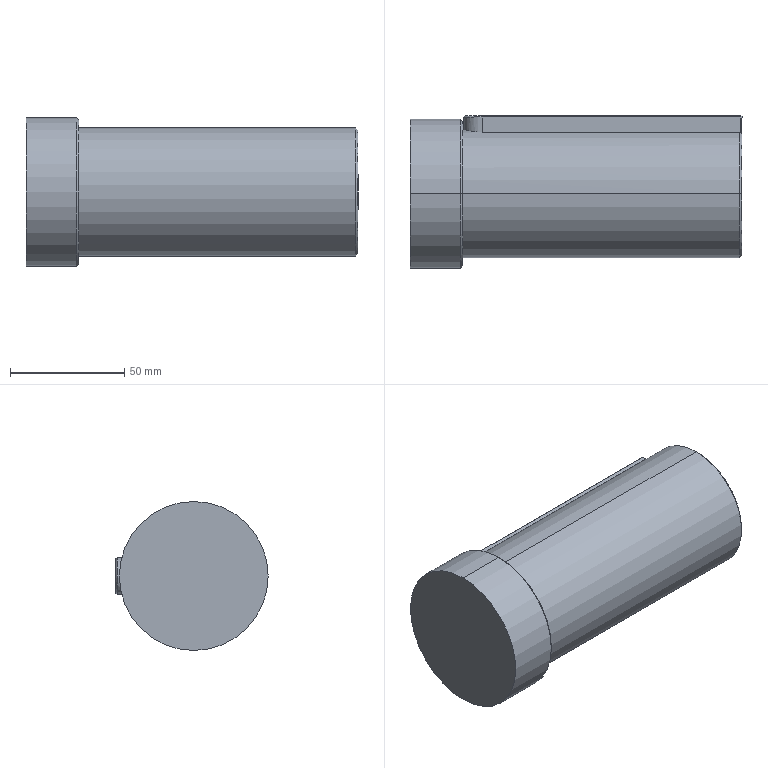Part | SolidWorks | features BaseBody 1 | 1 solid | 24 faces | box 145 x 66.5 x 65 mm | volume 388822 mm3 | plane 13 | cone 6 | cylinder 5 | commonest cylinder face diameters 56 x2 65 x2 16 x1
STEP:
#1=CARTESIAN_POINT('',(423.973,14.15,-28.));
#2=VERTEX_POINT('',#1);
#3=CARTESIAN_POINT('',(423.973,14.15,28.));
#4=VERTEX_POINT('',#3);
#5=CARTESIAN_POINT('',(423.973,14.15,0.));
#6=DIRECTION('',(1.,0.,0.));
#7=DIRECTION('',(0.,0.,-1.));
#8=AXIS2_PLACEMENT_3D('',#5,#6,#7);
#9=CIRCLE('',#8,28.);
#10=EDGE_CURVE('',#2,#4,#9,.T.);
#11=ORIENTED_EDGE('',*,*,#10,.T.);
#12=CARTESIAN_POINT('',(544.973,14.15,28.));
#13=VERTEX_POINT('',#12);
#14=CARTESIAN_POINT('',(484.973,14.15,28.));
#15=DIRECTION('',(1.,0.,0.));
#16=VECTOR('',#15,1000.);
#17=LINE('',#14,#16);
#18=EDGE_CURVE('',#4,#13,#17,.T.);
#19=ORIENTED_EDGE('',*,*,#18,.T.);
#20=CARTESIAN_POINT('',(544.973,40.983,8.));
#21=VERTEX_POINT('',#20);
#22=CARTESIAN_POINT('',(544.973,14.15,0.));
#23=DIRECTION('',(-1.,0.,0.));
#24=DIRECTION('',(0.,0.,-1.));
#25=AXIS2_PLACEMENT_3D('',#22,#23,#24);
#26=CIRCLE('',#25,28.);
#27=EDGE_CURVE('',#13,#21,#26,.T.);
#28=ORIENTED_EDGE('',*,*,#27,.T.);
#29=CARTESIAN_POINT('',(432.473,40.983,8.));
#30=VERTEX_POINT('',#29);
#31=CARTESIAN_POINT('',(484.973,40.983,8.));
#32=DIRECTION('',(-1.,0.,0.));
#33=VECTOR('',#32,1000.);
#34=LINE('',#31,#33);
#35=EDGE_CURVE('',#21,#30,#34,.T.);
#36=ORIENTED_EDGE('',*,*,#35,.T.);
#37=CARTESIAN_POINT('',(432.473,40.983,-8.));
#38=VERTEX_POINT('',#37);
#39=CARTESIAN_POINT('',(432.473,40.983,8.));
#40=CARTESIAN_POINT('',(431.941,40.983,8.));
#41=CARTESIAN_POINT('',(431.419,40.999,7.948));
#42=CARTESIAN_POINT('',(430.65,41.044,7.794));
#43=CARTESIAN_POINT('',(430.396,41.062,7.73));
#44=CARTESIAN_POINT('',(429.892,41.106,7.577));
#45=CARTESIAN_POINT('',(429.642,41.131,7.487));
#46=CARTESIAN_POINT('',(428.917,41.214,7.185));
#47=CARTESIAN_POINT('',(428.459,41.278,6.94));
#48=CARTESIAN_POINT('',(427.808,41.385,6.505));
#49=CARTESIAN_POINT('',(427.596,41.422,6.347));
#50=CARTESIAN_POINT('',(427.192,41.497,6.015));
#51=CARTESIAN_POINT('',(426.999,41.535,5.841));
#52=CARTESIAN_POINT('',(426.449,41.649,5.29));
#53=CARTESIAN_POINT('',(426.119,41.724,4.89));
#54=CARTESIAN_POINT('',(425.534,41.864,4.016));
#55=CARTESIAN_POINT('',(425.287,41.928,3.555));
#56=CARTESIAN_POINT('',(424.987,42.008,2.834));
#57=CARTESIAN_POINT('',(424.898,42.032,2.589));
#58=CARTESIAN_POINT('',(424.745,42.074,2.087));
#59=CARTESIAN_POINT('',(424.68,42.092,1.829));
#60=CARTESIAN_POINT('',(424.525,42.135,1.053));
#61=CARTESIAN_POINT('',(424.473,42.15,0.5324));
#62=CARTESIAN_POINT('',(424.472,42.151,-0.5171));
#63=CARTESIAN_POINT('',(424.525,42.135,-1.05));
#64=CARTESIAN_POINT('',(424.73,42.078,-2.078));
#65=CARTESIAN_POINT('',(424.881,42.036,-2.579));
#66=CARTESIAN_POINT('',(425.184,41.955,-3.308));
#67=CARTESIAN_POINT('',(425.297,41.926,-3.547));
#68=CARTESIAN_POINT('',(425.544,41.863,-4.007));
#69=CARTESIAN_POINT('',(425.678,41.83,-4.231));
#70=CARTESIAN_POINT('',(425.967,41.76,-4.662));
#71=CARTESIAN_POINT('',(426.121,41.724,-4.871));
#72=CARTESIAN_POINT('',(426.452,41.65,-5.275));
#73=CARTESIAN_POINT('',(426.629,41.612,-5.47));
#74=CARTESIAN_POINT('',(427.183,41.497,-6.025));
#75=CARTESIAN_POINT('',(427.584,41.422,-6.354));
#76=CARTESIAN_POINT('',(428.447,41.28,-6.933));
#77=CARTESIAN_POINT('',(428.916,41.214,-7.185));
#78=CARTESIAN_POINT('',(429.879,41.104,-7.586));
#79=CARTESIAN_POINT('',(430.378,41.06,-7.739));
#80=CARTESIAN_POINT('',(431.152,41.015,-7.895));
#81=CARTESIAN_POINT('',(431.415,41.003,-7.934));
#82=CARTESIAN_POINT('',(431.942,40.987,-7.987));
#83=CARTESIAN_POINT('',(432.207,40.983,-8.));
#84=CARTESIAN_POINT('',(432.473,40.983,-8.));
#85=B_SPLINE_CURVE_WITH_KNOTS('',3,(#39,#40,#41,#42,#43,#44,#45,#46,#47,#48,#49,#50,#51,#52,#53,#54,#55,#56,#57,#58,#59,#60,#61,#62,#63,#64,#65,#66,#67,#68,#69,#70,#71,#72,#73,#74,#75,#76,#77,#78,#79,#80,#81,#82,#83,#84),.UNSPECIFIED.,.F.,.F.,(4,2,2,2,2,2,2,2,2,2,2,2,2,2,2,2,2,2,2,2,2,2,4),(0.,0.001571,0.002356,0.003142,0.004713,0.005498,0.006284,0.007855,0.009425,0.01021,0.011,0.01257,0.01414,0.01571,0.01649,0.01728,0.01807,0.01885,0.02042,0.02199,0.02356,0.02435,0.02513),.UNSPECIFIED.);
#86=EDGE_CURVE('',#30,#38,#85,.T.);
#87=ORIENTED_EDGE('',*,*,#86,.T.);
#88=CARTESIAN_POINT('',(544.973,40.983,-8.));
#89=VERTEX_POINT('',#88);
#90=CARTESIAN_POINT('',(484.973,40.983,-8.));
#91=DIRECTION('',(1.,0.,0.));
#92=VECTOR('',#91,1000.);
#93=LINE('',#90,#92);
#94=EDGE_CURVE('',#38,#89,#93,.T.);
#95=ORIENTED_EDGE('',*,*,#94,.T.);
#96=CARTESIAN_POINT('',(544.973,14.15,-28.));
#97=VERTEX_POINT('',#96);
#98=CARTESIAN_POINT('',(544.973,14.15,0.));
#99=DIRECTION('',(-1.,0.,0.));
#100=DIRECTION('',(0.,0.,-1.));
#101=AXIS2_PLACEMENT_3D('',#98,#99,#100);
#102=CIRCLE('',#101,28.);
#103=EDGE_CURVE('',#89,#97,#102,.T.);
#104=ORIENTED_EDGE('',*,*,#103,.T.);
#105=CARTESIAN_POINT('',(484.973,14.15,-28.));
#106=DIRECTION('',(1.,0.,0.));
#107=VECTOR('',#106,1000.);
#108=LINE('',#105,#107);
#109=EDGE_CURVE('',#2,#97,#108,.T.);
#110=ORIENTED_EDGE('',*,*,#109,.F.);
#111=EDGE_LOOP('',(#11,#19,#28,#36,#87,#95,#104,#110));
#112=FACE_OUTER_BOUND('',#111,.T.);
#113=CARTESIAN_POINT('',(484.973,14.15,0.));
#114=DIRECTION('',(1.,0.,0.));
#115=DIRECTION('',(0.,0.,-1.));
#116=AXIS2_PLACEMENT_3D('',#113,#114,#115);
#117=CYLINDRICAL_SURFACE('',#116,28.);
#118=ADVANCED_FACE('',(#112),#117,.T.);
#119=CARTESIAN_POINT('',(545.973,40.088,-7.5));
#120=VERTEX_POINT('',#119);
#121=CARTESIAN_POINT('',(545.973,14.15,-27.));
#122=VERTEX_POINT('',#121);
#123=CARTESIAN_POINT('',(545.973,14.15,0.));
#124=DIRECTION('',(-1.,0.,0.));
#125=DIRECTION('',(0.,0.,1.));
#126=AXIS2_PLACEMENT_3D('',#123,#124,#125);
#127=CIRCLE('',#126,27.);
#128=EDGE_CURVE('',#120,#122,#127,.T.);
#129=ORIENTED_EDGE('',*,*,#128,.T.);
#130=CARTESIAN_POINT('',(544.973,14.15,-28.));
#131=DIRECTION('',(-0.7071,0.,-0.7071));
#132=VECTOR('',#131,1000.);
#133=LINE('',#130,#132);
#134=EDGE_CURVE('',#122,#97,#133,.T.);
#135=ORIENTED_EDGE('',*,*,#134,.T.);
#136=ORIENTED_EDGE('',*,*,#103,.F.);
#137=CARTESIAN_POINT('',(545.473,40.461,-8.));
#138=VERTEX_POINT('',#137);
#139=CARTESIAN_POINT('',(545.473,40.461,-8.));
#140=CARTESIAN_POINT('',(545.306,40.635,-8.));
#141=CARTESIAN_POINT('',(545.139,40.809,-8.));
#142=CARTESIAN_POINT('',(544.973,40.983,-8.));
#143=B_SPLINE_CURVE_WITH_KNOTS('',3,(#139,#140,#141,#142),.UNSPECIFIED.,.F.,.F.,(4,4),(0.,0.000723),.UNSPECIFIED.);
#144=EDGE_CURVE('',#138,#89,#143,.T.);
#145=ORIENTED_EDGE('',*,*,#144,.F.);
#146=CARTESIAN_POINT('',(545.473,40.461,-8.));
#147=CARTESIAN_POINT('',(545.64,40.337,-7.833));
#148=CARTESIAN_POINT('',(545.806,40.213,-7.666));
#149=CARTESIAN_POINT('',(545.973,40.088,-7.5));
#150=B_SPLINE_CURVE_WITH_KNOTS('',3,(#146,#147,#148,#149),.UNSPECIFIED.,.F.,.F.,(4,4),(0.,0.0007996),.UNSPECIFIED.);
#151=EDGE_CURVE('',#138,#120,#150,.T.);
#152=ORIENTED_EDGE('',*,*,#151,.T.);
#153=EDGE_LOOP('',(#129,#135,#136,#145,#152));
#154=FACE_OUTER_BOUND('',#153,.T.);
#155=CARTESIAN_POINT('',(544.973,14.15,0.));
#156=DIRECTION('',(-1.,0.,0.));
#157=DIRECTION('',(0.,0.,1.));
#158=AXIS2_PLACEMENT_3D('',#155,#156,#157);
#159=CONICAL_SURFACE('',#158,28.,0.7854);
#160=ADVANCED_FACE('',(#154),#159,.T.);
#161=ORIENTED_EDGE('',*,*,#134,.F.);
#162=CARTESIAN_POINT('',(545.973,14.15,27.));
#163=VERTEX_POINT('',#162);
#164=CARTESIAN_POINT('',(545.973,14.15,0.));
#165=DIRECTION('',(-1.,0.,0.));
#166=DIRECTION('',(0.,0.,1.));
#167=AXIS2_PLACEMENT_3D('',#164,#165,#166);
#168=CIRCLE('',#167,27.);
#169=EDGE_CURVE('',#122,#163,#168,.T.);
#170=ORIENTED_EDGE('',*,*,#169,.T.);
#171=CARTESIAN_POINT('',(544.973,14.15,28.));
#172=DIRECTION('',(-0.7071,0.,0.7071));
#173=VECTOR('',#172,1000.);
#174=LINE('',#171,#173);
#175=EDGE_CURVE('',#163,#13,#174,.T.);
#176=ORIENTED_EDGE('',*,*,#175,.T.);
#177=CARTESIAN_POINT('',(544.973,14.15,0.));
#178=DIRECTION('',(-1.,0.,0.));
#179=DIRECTION('',(0.,0.,-1.));
#180=AXIS2_PLACEMENT_3D('',#177,#178,#179);
#181=CIRCLE('',#180,28.);
#182=EDGE_CURVE('',#97,#13,#181,.T.);
#183=ORIENTED_EDGE('',*,*,#182,.F.);
#184=EDGE_LOOP('',(#161,#170,#176,#183));
#185=FACE_OUTER_BOUND('',#184,.T.);
#186=CARTESIAN_POINT('',(544.973,14.15,0.));
#187=DIRECTION('',(-1.,0.,0.));
#188=DIRECTION('',(0.,0.,1.));
#189=AXIS2_PLACEMENT_3D('',#186,#187,#188);
#190=CONICAL_SURFACE('',#189,28.,0.7854);
#191=ADVANCED_FACE('',(#185),#190,.T.);
#192=CARTESIAN_POINT('',(423.973,14.15,-31.5));
#193=VERTEX_POINT('',#192);
#194=CARTESIAN_POINT('',(423.973,14.15,31.5));
#195=VERTEX_POINT('',#194);
#196=CARTESIAN_POINT('',(423.973,14.15,0.));
#197=DIRECTION('',(1.,0.,0.));
#198=DIRECTION('',(0.,0.,1.));
#199=AXIS2_PLACEMENT_3D('',#196,#197,#198);
#200=CIRCLE('',#199,31.5);
#201=EDGE_CURVE('',#193,#195,#200,.T.);
#202=ORIENTED_EDGE('',*,*,#201,.F.);
#203=CARTESIAN_POINT('',(422.973,14.15,-32.5));
#204=VERTEX_POINT('',#203);
#205=CARTESIAN_POINT('',(422.973,14.15,-32.5));
#206=DIRECTION('',(-0.7071,0.,-0.7071));
#207=VECTOR('',#206,1000.);
#208=LINE('',#205,#207);
#209=EDGE_CURVE('',#193,#204,#208,.T.);
#210=ORIENTED_EDGE('',*,*,#209,.T.);
#211=CARTESIAN_POINT('',(422.973,14.15,32.5));
#212=VERTEX_POINT('',#211);
#213=CARTESIAN_POINT('',(422.973,14.15,0.));
#214=DIRECTION('',(1.,0.,0.));
#215=DIRECTION('',(0.,-1.,0.));
#216=AXIS2_PLACEMENT_3D('',#213,#214,#215);
#217=CIRCLE('',#216,32.5);
#218=EDGE_CURVE('',#204,#212,#217,.T.);
#219=ORIENTED_EDGE('',*,*,#218,.T.);
#220=CARTESIAN_POINT('',(422.973,14.15,32.5));
#221=DIRECTION('',(-0.7071,0.,0.7071));
#222=VECTOR('',#221,1000.);
#223=LINE('',#220,#222);
#224=EDGE_CURVE('',#195,#212,#223,.T.);
#225=ORIENTED_EDGE('',*,*,#224,.F.);
#226=EDGE_LOOP('',(#202,#210,#219,#225));
#227=FACE_OUTER_BOUND('',#226,.T.);
#228=CARTESIAN_POINT('',(422.973,14.15,0.));
#229=DIRECTION('',(-1.,0.,0.));
#230=DIRECTION('',(0.,0.,1.));
#231=AXIS2_PLACEMENT_3D('',#228,#229,#230);
#232=CONICAL_SURFACE('',#231,32.5,0.7854);
#233=ADVANCED_FACE('',(#227),#232,.T.);
#234=CARTESIAN_POINT('',(400.973,14.15,-32.5));
#235=VERTEX_POINT('',#234);
#236=CARTESIAN_POINT('',(400.973,14.15,32.5));
#237=VERTEX_POINT('',#236);
#238=CARTESIAN_POINT('',(400.973,14.15,0.));
#239=DIRECTION('',(1.,0.,0.));
#240=DIRECTION('',(0.,0.,-1.));
#241=AXIS2_PLACEMENT_3D('',#238,#239,#240);
#242=CIRCLE('',#241,32.5);
#243=EDGE_CURVE('',#235,#237,#242,.T.);
#244=ORIENTED_EDGE('',*,*,#243,.T.);
#245=CARTESIAN_POINT('',(412.473,14.15,32.5));
#246=DIRECTION('',(1.,0.,0.));
#247=VECTOR('',#246,1000.);
#248=LINE('',#245,#247);
#249=EDGE_CURVE('',#237,#212,#248,.T.);
#250=ORIENTED_EDGE('',*,*,#249,.T.);
#251=ORIENTED_EDGE('',*,*,#218,.F.);
#252=CARTESIAN_POINT('',(412.473,14.15,-32.5));
#253=DIRECTION('',(1.,0.,0.));
#254=VECTOR('',#253,1000.);
#255=LINE('',#252,#254);
#256=EDGE_CURVE('',#235,#204,#255,.T.);
#257=ORIENTED_EDGE('',*,*,#256,.F.);
#258=EDGE_LOOP('',(#244,#250,#251,#257));
#259=FACE_OUTER_BOUND('',#258,.T.);
#260=CARTESIAN_POINT('',(412.473,14.15,0.));
#261=DIRECTION('',(1.,0.,0.));
#262=DIRECTION('',(0.,0.,-1.));
#263=AXIS2_PLACEMENT_3D('',#260,#261,#262);
#264=CYLINDRICAL_SURFACE('',#263,32.5);
#265=ADVANCED_FACE('',(#259),#264,.T.);
#266=ORIENTED_EDGE('',*,*,#18,.F.);
#267=CARTESIAN_POINT('',(423.973,14.15,0.));
#268=DIRECTION('',(1.,0.,0.));
#269=DIRECTION('',(0.,0.,-1.));
#270=AXIS2_PLACEMENT_3D('',#267,#268,#269);
#271=CIRCLE('',#270,28.);
#272=EDGE_CURVE('',#4,#2,#271,.T.);
#273=ORIENTED_EDGE('',*,*,#272,.T.);
#274=ORIENTED_EDGE('',*,*,#109,.T.);
#275=ORIENTED_EDGE('',*,*,#182,.T.);
#276=EDGE_LOOP('',(#266,#273,#274,#275));
#277=FACE_OUTER_BOUND('',#276,.T.);
#278=CARTESIAN_POINT('',(484.973,14.15,0.));
#279=DIRECTION('',(1.,0.,0.));
#280=DIRECTION('',(0.,0.,-1.));
#281=AXIS2_PLACEMENT_3D('',#278,#279,#280);
#282=CYLINDRICAL_SURFACE('',#281,28.);
#283=ADVANCED_FACE('',(#277),#282,.T.);
#284=ORIENTED_EDGE('',*,*,#10,.F.);
#285=ORIENTED_EDGE('',*,*,#272,.F.);
#286=EDGE_LOOP('',(#284,#285));
#287=FACE_BOUND('',#286,.T.);
#288=CARTESIAN_POINT('',(423.973,14.15,0.));
#289=DIRECTION('',(1.,0.,0.));
#290=DIRECTION('',(0.,0.,1.));
#291=AXIS2_PLACEMENT_3D('',#288,#289,#290);
#292=CIRCLE('',#291,31.5);
#293=EDGE_CURVE('',#195,#193,#292,.T.);
#294=ORIENTED_EDGE('',*,*,#293,.T.);
#295=ORIENTED_EDGE('',*,*,#201,.T.);
#296=EDGE_LOOP('',(#294,#295));
#297=FACE_OUTER_BOUND('',#296,.T.);
#298=CARTESIAN_POINT('',(423.973,44.4,0.));
#299=DIRECTION('',(1.,0.,0.));
#300=DIRECTION('',(0.,0.,-1.));
#301=AXIS2_PLACEMENT_3D('',#298,#299,#300);
#302=PLANE('',#301);
#303=ADVANCED_FACE('',(#287,#297),#302,.T.);
#304=CARTESIAN_POINT('',(432.473,47.65,-8.));
#305=VERTEX_POINT('',#304);
#306=CARTESIAN_POINT('',(432.473,42.15,-8.));
#307=DIRECTION('',(0.,1.,0.));
#308=VECTOR('',#307,1000.);
#309=LINE('',#306,#308);
#310=EDGE_CURVE('',#38,#305,#309,.T.);
#311=ORIENTED_EDGE('',*,*,#310,.T.);
#312=CARTESIAN_POINT('',(545.473,47.65,-8.));
#313=VERTEX_POINT('',#312);
#314=CARTESIAN_POINT('',(432.473,47.65,-8.));
#315=DIRECTION('',(1.,0.,0.));
#316=VECTOR('',#315,1000.);
#317=LINE('',#314,#316);
#318=EDGE_CURVE('',#305,#313,#317,.T.);
#319=ORIENTED_EDGE('',*,*,#318,.T.);
#320=CARTESIAN_POINT('',(545.473,42.15,-8.));
#321=DIRECTION('',(0.,-1.,0.));
#322=VECTOR('',#321,1000.);
#323=LINE('',#320,#322);
#324=EDGE_CURVE('',#313,#138,#323,.T.);
#325=ORIENTED_EDGE('',*,*,#324,.T.);
#326=ORIENTED_EDGE('',*,*,#144,.T.);
#327=ORIENTED_EDGE('',*,*,#94,.F.);
#328=EDGE_LOOP('',(#311,#319,#325,#326,#327));
#329=FACE_OUTER_BOUND('',#328,.T.);
#330=CARTESIAN_POINT('',(432.473,42.15,-8.));
#331=DIRECTION('',(0.,0.,-1.));
#332=DIRECTION('',(-1.,0.,0.));
#333=AXIS2_PLACEMENT_3D('',#330,#331,#332);
#334=PLANE('',#333);
#335=ADVANCED_FACE('',(#329),#334,.T.);
#336=ORIENTED_EDGE('',*,*,#86,.F.);
#337=CARTESIAN_POINT('',(432.473,47.65,8.));
#338=VERTEX_POINT('',#337);
#339=CARTESIAN_POINT('',(432.473,42.15,8.));
#340=DIRECTION('',(0.,1.,0.));
#341=VECTOR('',#340,1000.);
#342=LINE('',#339,#341);
#343=EDGE_CURVE('',#30,#338,#342,.T.);
#344=ORIENTED_EDGE('',*,*,#343,.T.);
#345=CARTESIAN_POINT('',(432.473,47.65,0.));
#346=DIRECTION('',(0.,-1.,0.));
#347=DIRECTION('',(0.,0.,1.));
#348=AXIS2_PLACEMENT_3D('',#345,#346,#347);
#349=CIRCLE('',#348,8.);
#350=EDGE_CURVE('',#338,#305,#349,.T.);
#351=ORIENTED_EDGE('',*,*,#350,.T.);
#352=ORIENTED_EDGE('',*,*,#310,.F.);
#353=EDGE_LOOP('',(#336,#344,#351,#352));
#354=FACE_OUTER_BOUND('',#353,.T.);
#355=CARTESIAN_POINT('',(432.473,42.15,0.));
#356=DIRECTION('',(0.,1.,0.));
#357=DIRECTION('',(0.,0.,1.));
#358=AXIS2_PLACEMENT_3D('',#355,#356,#357);
#359=CYLINDRICAL_SURFACE('',#358,8.);
#360=ADVANCED_FACE('',(#354),#359,.T.);
#361=ORIENTED_EDGE('',*,*,#35,.F.);
#362=CARTESIAN_POINT('',(545.473,40.461,8.));
#363=VERTEX_POINT('',#362);
#364=CARTESIAN_POINT('',(544.973,40.983,8.));
#365=CARTESIAN_POINT('',(545.139,40.809,8.));
#366=CARTESIAN_POINT('',(545.306,40.635,8.));
#367=CARTESIAN_POINT('',(545.473,40.461,8.));
#368=B_SPLINE_CURVE_WITH_KNOTS('',3,(#364,#365,#366,#367),.UNSPECIFIED.,.F.,.F.,(4,4),(0.,0.000723),.UNSPECIFIED.);
#369=EDGE_CURVE('',#21,#363,#368,.T.);
#370=ORIENTED_EDGE('',*,*,#369,.T.);
#371=CARTESIAN_POINT('',(545.473,47.65,8.));
#372=VERTEX_POINT('',#371);
#373=CARTESIAN_POINT('',(545.473,42.15,8.));
#374=DIRECTION('',(0.,1.,0.));
#375=VECTOR('',#374,1000.);
#376=LINE('',#373,#375);
#377=EDGE_CURVE('',#363,#372,#376,.T.);
#378=ORIENTED_EDGE('',*,*,#377,.T.);
#379=CARTESIAN_POINT('',(545.973,47.65,8.));
#380=DIRECTION('',(-1.,0.,0.));
#381=VECTOR('',#380,1000.);
#382=LINE('',#379,#381);
#383=EDGE_CURVE('',#372,#338,#382,.T.);
#384=ORIENTED_EDGE('',*,*,#383,.T.);
#385=ORIENTED_EDGE('',*,*,#343,.F.);
#386=EDGE_LOOP('',(#361,#370,#378,#384,#385));
#387=FACE_OUTER_BOUND('',#386,.T.);
#388=CARTESIAN_POINT('',(545.973,42.15,8.));
#389=DIRECTION('',(0.,0.,1.));
#390=DIRECTION('',(1.,0.,0.));
#391=AXIS2_PLACEMENT_3D('',#388,#389,#390);
#392=PLANE('',#391);
#393=ADVANCED_FACE('',(#387),#392,.T.);
#394=ORIENTED_EDGE('',*,*,#175,.F.);
#395=CARTESIAN_POINT('',(545.973,40.088,7.5));
#396=VERTEX_POINT('',#395);
#397=CARTESIAN_POINT('',(545.973,14.15,0.));
#398=DIRECTION('',(-1.,0.,0.));
#399=DIRECTION('',(0.,0.,1.));
#400=AXIS2_PLACEMENT_3D('',#397,#398,#399);
#401=CIRCLE('',#400,27.);
#402=EDGE_CURVE('',#163,#396,#401,.T.);
#403=ORIENTED_EDGE('',*,*,#402,.T.);
#404=CARTESIAN_POINT('',(545.973,40.088,7.5));
#405=CARTESIAN_POINT('',(545.806,40.213,7.666));
#406=CARTESIAN_POINT('',(545.64,40.337,7.833));
#407=CARTESIAN_POINT('',(545.473,40.461,8.));
#408=B_SPLINE_CURVE_WITH_KNOTS('',3,(#404,#405,#406,#407),.UNSPECIFIED.,.F.,.F.,(4,4),(0.,0.0007996),.UNSPECIFIED.);
#409=EDGE_CURVE('',#396,#363,#408,.T.);
#410=ORIENTED_EDGE('',*,*,#409,.T.);
#411=ORIENTED_EDGE('',*,*,#369,.F.);
#412=ORIENTED_EDGE('',*,*,#27,.F.);
#413=EDGE_LOOP('',(#394,#403,#410,#411,#412));
#414=FACE_OUTER_BOUND('',#413,.T.);
#415=CARTESIAN_POINT('',(544.973,14.15,0.));
#416=DIRECTION('',(-1.,0.,0.));
#417=DIRECTION('',(0.,0.,1.));
#418=AXIS2_PLACEMENT_3D('',#415,#416,#417);
#419=CONICAL_SURFACE('',#418,28.,0.7854);
#420=ADVANCED_FACE('',(#414),#419,.T.);
#421=ORIENTED_EDGE('',*,*,#209,.F.);
#422=ORIENTED_EDGE('',*,*,#293,.F.);
#423=ORIENTED_EDGE('',*,*,#224,.T.);
#424=CARTESIAN_POINT('',(422.973,14.15,0.));
#425=DIRECTION('',(1.,0.,0.));
#426=DIRECTION('',(0.,-1.,0.));
#427=AXIS2_PLACEMENT_3D('',#424,#425,#426);
#428=CIRCLE('',#427,32.5);
#429=EDGE_CURVE('',#212,#204,#428,.T.);
#430=ORIENTED_EDGE('',*,*,#429,.T.);
#431=EDGE_LOOP('',(#421,#422,#423,#430));
#432=FACE_OUTER_BOUND('',#431,.T.);
#433=CARTESIAN_POINT('',(422.973,14.15,0.));
#434=DIRECTION('',(-1.,0.,0.));
#435=DIRECTION('',(0.,0.,1.));
#436=AXIS2_PLACEMENT_3D('',#433,#434,#435);
#437=CONICAL_SURFACE('',#436,32.5,0.7854);
#438=ADVANCED_FACE('',(#432),#437,.T.);
#439=CARTESIAN_POINT('',(432.473,48.15,-7.5));
#440=VERTEX_POINT('',#439);
#441=CARTESIAN_POINT('',(432.473,47.9,-7.75));
#442=DIRECTION('',(0.,0.7071,0.7071));
#443=VECTOR('',#442,1000.);
#444=LINE('',#441,#443);
#445=EDGE_CURVE('',#305,#440,#444,.T.);
#446=ORIENTED_EDGE('',*,*,#445,.T.);
#447=CARTESIAN_POINT('',(545.473,48.15,-7.5));
#448=VERTEX_POINT('',#447);
#449=CARTESIAN_POINT('',(459.666,48.15,-7.5));
#450=DIRECTION('',(1.,0.,0.));
#451=VECTOR('',#450,1000.);
#452=LINE('',#449,#451);
#453=EDGE_CURVE('',#440,#448,#452,.T.);
#454=ORIENTED_EDGE('',*,*,#453,.T.);
#455=CARTESIAN_POINT('',(545.473,47.9,-7.75));
#456=DIRECTION('',(0.,-0.7071,-0.7071));
#457=VECTOR('',#456,1000.);
#458=LINE('',#455,#457);
#459=EDGE_CURVE('',#448,#313,#458,.T.);
#460=ORIENTED_EDGE('',*,*,#459,.T.);
#461=ORIENTED_EDGE('',*,*,#318,.F.);
#462=EDGE_LOOP('',(#446,#454,#460,#461));
#463=FACE_OUTER_BOUND('',#462,.T.);
#464=CARTESIAN_POINT('',(459.666,47.9,-7.75));
#465=DIRECTION('',(0.,0.7071,-0.7071));
#466=DIRECTION('',(0.,0.7071,0.7071));
#467=AXIS2_PLACEMENT_3D('',#464,#465,#466);
#468=PLANE('',#467);
#469=ADVANCED_FACE('',(#463),#468,.T.);
#470=CARTESIAN_POINT('',(545.973,47.65,-7.5));
#471=VERTEX_POINT('',#470);
#472=CARTESIAN_POINT('',(545.723,47.65,-7.75));
#473=DIRECTION('',(0.7071,0.,0.7071));
#474=VECTOR('',#473,1000.);
#475=LINE('',#472,#474);
#476=EDGE_CURVE('',#313,#471,#475,.T.);
#477=ORIENTED_EDGE('',*,*,#476,.T.);
#478=CARTESIAN_POINT('',(545.973,35.15,-7.5));
#479=DIRECTION('',(0.,-1.,0.));
#480=VECTOR('',#479,1000.);
#481=LINE('',#478,#480);
#482=EDGE_CURVE('',#471,#120,#481,.T.);
#483=ORIENTED_EDGE('',*,*,#482,.T.);
#484=ORIENTED_EDGE('',*,*,#151,.F.);
#485=ORIENTED_EDGE('',*,*,#324,.F.);
#486=EDGE_LOOP('',(#477,#483,#484,#485));
#487=FACE_OUTER_BOUND('',#486,.T.);
#488=CARTESIAN_POINT('',(545.723,35.15,-7.75));
#489=DIRECTION('',(0.7071,0.,-0.7071));
#490=DIRECTION('',(-0.7071,0.,-0.7071));
#491=AXIS2_PLACEMENT_3D('',#488,#489,#490);
#492=PLANE('',#491);
#493=ADVANCED_FACE('',(#487),#492,.T.);
#494=CARTESIAN_POINT('',(432.473,48.15,7.5));
#495=VERTEX_POINT('',#494);
#496=CARTESIAN_POINT('',(432.473,47.9,7.75));
#497=DIRECTION('',(0.,0.7071,-0.7071));
#498=VECTOR('',#497,1000.);
#499=LINE('',#496,#498);
#500=EDGE_CURVE('',#338,#495,#499,.T.);
#501=ORIENTED_EDGE('',*,*,#500,.T.);
#502=CARTESIAN_POINT('',(432.473,48.15,0.));
#503=DIRECTION('',(0.,-1.,0.));
#504=DIRECTION('',(0.,0.,-1.));
#505=AXIS2_PLACEMENT_3D('',#502,#503,#504);
#506=CIRCLE('',#505,7.5);
#507=EDGE_CURVE('',#495,#440,#506,.T.);
#508=ORIENTED_EDGE('',*,*,#507,.T.);
#509=ORIENTED_EDGE('',*,*,#445,.F.);
#510=ORIENTED_EDGE('',*,*,#350,.F.);
#511=EDGE_LOOP('',(#501,#508,#509,#510));
#512=FACE_OUTER_BOUND('',#511,.T.);
#513=CARTESIAN_POINT('',(432.473,47.65,0.));
#514=DIRECTION('',(0.,-1.,0.));
#515=DIRECTION('',(0.,0.,-1.));
#516=AXIS2_PLACEMENT_3D('',#513,#514,#515);
#517=CONICAL_SURFACE('',#516,8.,0.7854);
#518=ADVANCED_FACE('',(#512),#517,.T.);
#519=CARTESIAN_POINT('',(545.473,48.15,7.5));
#520=VERTEX_POINT('',#519);
#521=CARTESIAN_POINT('',(545.473,47.9,7.75));
#522=DIRECTION('',(0.,0.7071,-0.7071));
#523=VECTOR('',#522,1000.);
#524=LINE('',#521,#523);
#525=EDGE_CURVE('',#372,#520,#524,.T.);
#526=ORIENTED_EDGE('',*,*,#525,.T.);
#527=CARTESIAN_POINT('',(516.416,48.15,7.5));
#528=DIRECTION('',(-1.,0.,0.));
#529=VECTOR('',#528,1000.);
#530=LINE('',#527,#529);
#531=EDGE_CURVE('',#520,#495,#530,.T.);
#532=ORIENTED_EDGE('',*,*,#531,.T.);
#533=ORIENTED_EDGE('',*,*,#500,.F.);
#534=ORIENTED_EDGE('',*,*,#383,.F.);
#535=EDGE_LOOP('',(#526,#532,#533,#534));
#536=FACE_OUTER_BOUND('',#535,.T.);
#537=CARTESIAN_POINT('',(516.416,47.9,7.75));
#538=DIRECTION('',(0.,0.7071,0.7071));
#539=DIRECTION('',(0.,-0.7071,0.7071));
#540=AXIS2_PLACEMENT_3D('',#537,#538,#539);
#541=PLANE('',#540);
#542=ADVANCED_FACE('',(#536),#541,.T.);
#543=CARTESIAN_POINT('',(545.973,47.65,7.5));
#544=VERTEX_POINT('',#543);
#545=CARTESIAN_POINT('',(545.723,47.65,7.75));
#546=DIRECTION('',(-0.7071,0.,0.7071));
#547=VECTOR('',#546,1000.);
#548=LINE('',#545,#547);
#549=EDGE_CURVE('',#544,#372,#548,.T.);
#550=ORIENTED_EDGE('',*,*,#549,.T.);
#551=ORIENTED_EDGE('',*,*,#377,.F.);
#552=ORIENTED_EDGE('',*,*,#409,.F.);
#553=CARTESIAN_POINT('',(545.973,35.15,7.5));
#554=DIRECTION('',(0.,1.,0.));
#555=VECTOR('',#554,1000.);
#556=LINE('',#553,#555);
#557=EDGE_CURVE('',#396,#544,#556,.T.);
#558=ORIENTED_EDGE('',*,*,#557,.T.);
#559=EDGE_LOOP('',(#550,#551,#552,#558));
#560=FACE_OUTER_BOUND('',#559,.T.);
#561=CARTESIAN_POINT('',(545.723,35.15,7.75));
#562=DIRECTION('',(0.7071,0.,0.7071));
#563=DIRECTION('',(0.7071,0.,-0.7071));
#564=AXIS2_PLACEMENT_3D('',#561,#562,#563);
#565=PLANE('',#564);
#566=ADVANCED_FACE('',(#560),#565,.T.);
#567=CARTESIAN_POINT('',(545.973,47.65,0.));
#568=DIRECTION('',(0.,0.,1.));
#569=VECTOR('',#568,1000.);
#570=LINE('',#567,#569);
#571=EDGE_CURVE('',#471,#544,#570,.T.);
#572=ORIENTED_EDGE('',*,*,#571,.T.);
#573=ORIENTED_EDGE('',*,*,#557,.F.);
#574=ORIENTED_EDGE('',*,*,#402,.F.);
#575=ORIENTED_EDGE('',*,*,#169,.F.);
#576=ORIENTED_EDGE('',*,*,#128,.F.);
#577=ORIENTED_EDGE('',*,*,#482,.F.);
#578=EDGE_LOOP('',(#572,#573,#574,#575,#576,#577));
#579=FACE_OUTER_BOUND('',#578,.T.);
#580=CARTESIAN_POINT('',(545.973,28.15,0.));
#581=DIRECTION('',(1.,0.,0.));
#582=DIRECTION('',(0.,0.,-1.));
#583=AXIS2_PLACEMENT_3D('',#580,#581,#582);
#584=PLANE('',#583);
#585=ADVANCED_FACE('',(#579),#584,.T.);
#586=ORIENTED_EDGE('',*,*,#249,.F.);
#587=CARTESIAN_POINT('',(400.973,14.15,0.));
#588=DIRECTION('',(1.,0.,0.));
#589=DIRECTION('',(0.,0.,-1.));
#590=AXIS2_PLACEMENT_3D('',#587,#588,#589);
#591=CIRCLE('',#590,32.5);
#592=EDGE_CURVE('',#237,#235,#591,.T.);
#593=ORIENTED_EDGE('',*,*,#592,.T.);
#594=ORIENTED_EDGE('',*,*,#256,.T.);
#595=ORIENTED_EDGE('',*,*,#429,.F.);
#596=EDGE_LOOP('',(#586,#593,#594,#595));
#597=FACE_OUTER_BOUND('',#596,.T.);
#598=CARTESIAN_POINT('',(412.473,14.15,0.));
#599=DIRECTION('',(1.,0.,0.));
#600=DIRECTION('',(0.,0.,-1.));
#601=AXIS2_PLACEMENT_3D('',#598,#599,#600);
#602=CYLINDRICAL_SURFACE('',#601,32.5);
#603=ADVANCED_FACE('',(#597),#602,.T.);
#604=ORIENTED_EDGE('',*,*,#453,.F.);
#605=ORIENTED_EDGE('',*,*,#507,.F.);
#606=ORIENTED_EDGE('',*,*,#531,.F.);
#607=CARTESIAN_POINT('',(545.473,48.15,0.));
#608=DIRECTION('',(0.,0.,-1.));
#609=VECTOR('',#608,1000.);
#610=LINE('',#607,#609);
#611=EDGE_CURVE('',#520,#448,#610,.T.);
#612=ORIENTED_EDGE('',*,*,#611,.T.);
#613=EDGE_LOOP('',(#604,#605,#606,#612));
#614=FACE_OUTER_BOUND('',#613,.T.);
#615=CARTESIAN_POINT('',(486.859,48.15,0.));
#616=DIRECTION('',(0.,1.,0.));
#617=DIRECTION('',(-1.,0.,0.));
#618=AXIS2_PLACEMENT_3D('',#615,#616,#617);
#619=PLANE('',#618);
#620=ADVANCED_FACE('',(#614),#619,.T.);
#621=CARTESIAN_POINT('',(545.473,48.15,-7.5));
#622=DIRECTION('',(0.7071,-0.7071,0.));
#623=VECTOR('',#622,1000.);
#624=LINE('',#621,#623);
#625=EDGE_CURVE('',#448,#471,#624,.T.);
#626=ORIENTED_EDGE('',*,*,#625,.T.);
#627=ORIENTED_EDGE('',*,*,#476,.F.);
#628=ORIENTED_EDGE('',*,*,#459,.F.);
#629=EDGE_LOOP('',(#626,#627,#628));
#630=FACE_OUTER_BOUND('',#629,.T.);
#631=CARTESIAN_POINT('',(545.723,47.65,-7.75));
#632=DIRECTION('',(0.5774,0.5774,-0.5774));
#633=DIRECTION('',(-0.7071,0.,-0.7071));
#634=AXIS2_PLACEMENT_3D('',#631,#632,#633);
#635=PLANE('',#634);
#636=ADVANCED_FACE('',(#630),#635,.T.);
#637=ORIENTED_EDGE('',*,*,#525,.F.);
#638=ORIENTED_EDGE('',*,*,#549,.F.);
#639=CARTESIAN_POINT('',(545.973,47.65,7.5));
#640=DIRECTION('',(-0.7071,0.7071,0.));
#641=VECTOR('',#640,1000.);
#642=LINE('',#639,#641);
#643=EDGE_CURVE('',#544,#520,#642,.T.);
#644=ORIENTED_EDGE('',*,*,#643,.T.);
#645=EDGE_LOOP('',(#637,#638,#644));
#646=FACE_OUTER_BOUND('',#645,.T.);
#647=CARTESIAN_POINT('',(545.723,47.65,7.75));
#648=DIRECTION('',(0.5774,0.5774,0.5774));
#649=DIRECTION('',(0.7071,0.,-0.7071));
#650=AXIS2_PLACEMENT_3D('',#647,#648,#649);
#651=PLANE('',#650);
#652=ADVANCED_FACE('',(#646),#651,.T.);
#653=ORIENTED_EDGE('',*,*,#625,.F.);
#654=ORIENTED_EDGE('',*,*,#611,.F.);
#655=ORIENTED_EDGE('',*,*,#643,.F.);
#656=ORIENTED_EDGE('',*,*,#571,.F.);
#657=EDGE_LOOP('',(#653,#654,#655,#656));
#658=FACE_OUTER_BOUND('',#657,.T.);
#659=CARTESIAN_POINT('',(545.723,47.9,0.));
#660=DIRECTION('',(0.7071,0.7071,0.));
#661=DIRECTION('',(-0.7071,0.7071,0.));
#662=AXIS2_PLACEMENT_3D('',#659,#660,#661);
#663=PLANE('',#662);
#664=ADVANCED_FACE('',(#658),#663,.T.);
#665=ORIENTED_EDGE('',*,*,#243,.F.);
#666=ORIENTED_EDGE('',*,*,#592,.F.);
#667=EDGE_LOOP('',(#665,#666));
#668=FACE_OUTER_BOUND('',#667,.T.);
#669=CARTESIAN_POINT('',(400.973,30.4,0.));
#670=DIRECTION('',(-1.,0.,0.));
#671=DIRECTION('',(0.,0.,1.));
#672=AXIS2_PLACEMENT_3D('',#669,#670,#671);
#673=PLANE('',#672);
#674=ADVANCED_FACE('',(#668),#673,.T.);
#675=CLOSED_SHELL('',(#118,#160,#191,#233,#265,#283,#303,#335,#360,#393,#420,#438,#469,#493,#518,#542,#566,#585,#603,#620,#636,#652,#664,#674));
#676=MANIFOLD_SOLID_BREP('',#675);
#677=CARTESIAN_POINT('',(0.,0.,0.));
#678=DIRECTION('',(0.,0.,1.));
#679=DIRECTION('',(1.,0.,0.));
#680=AXIS2_PLACEMENT_3D('',#677,#678,#679);
#681=(LENGTH_UNIT()NAMED_UNIT(*)SI_UNIT(.MILLI.,.METRE.));
#682=UNCERTAINTY_MEASURE_WITH_UNIT(LENGTH_MEASURE(0.00001),#681,'','');
#683=(NAMED_UNIT(*)PLANE_ANGLE_UNIT()SI_UNIT($,.RADIAN.));
#684=(NAMED_UNIT(*)SI_UNIT($,.STERADIAN.)SOLID_ANGLE_UNIT());
#685=(GEOMETRIC_REPRESENTATION_CONTEXT(3)GLOBAL_UNCERTAINTY_ASSIGNED_CONTEXT((#682))GLOBAL_UNIT_ASSIGNED_CONTEXT((#681,#683,#684))REPRESENTATION_CONTEXT('',''));
#686=ADVANCED_BREP_SHAPE_REPRESENTATION('',(#676,#680),#685);